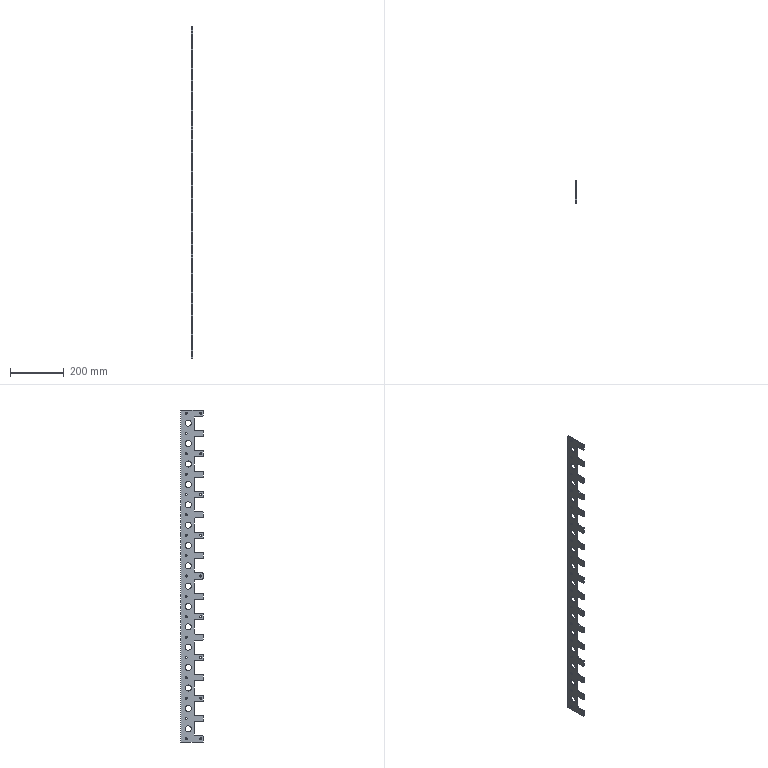Part | SolidWorks | features BaseBody 1, ICE 1 | 1 solid | 219 faces | box 4 x 85 x 1231 mm | volume 272752 mm3 | cylinder 149 | plane 70 | commonest cylinder face diameters 7.5 x52 8 x33 6 x32 22.61 x32